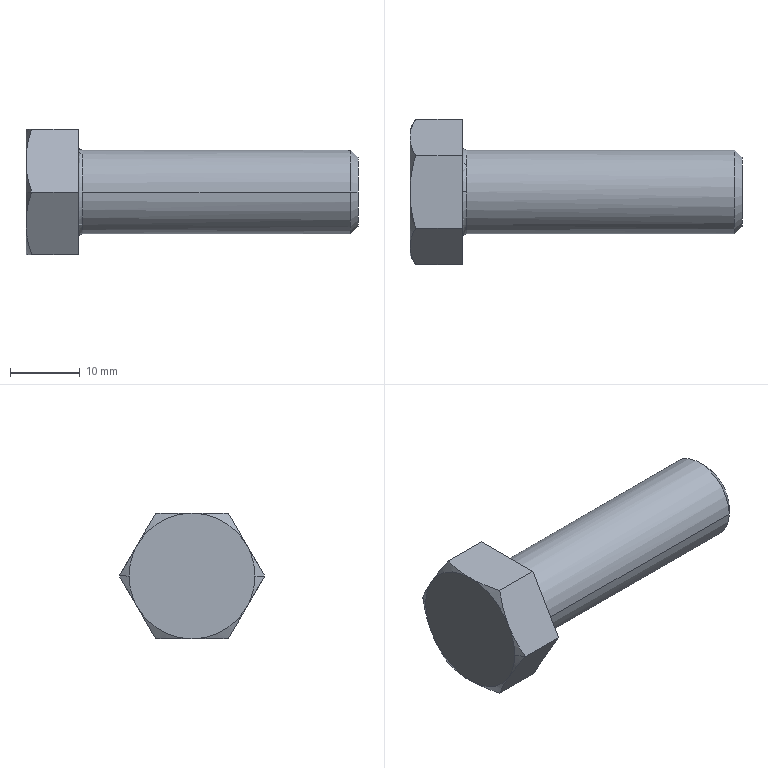Part | STEP file | KS B 1002 - C  M 12 x 40 | 1 solid | 23 faces | box 47.5 x 20.785 x 18 mm | volume 6605 mm3 | cone 10 | plane 9 | torus 2 | cylinder 2 | commonest cylinder face diameters 12 x2